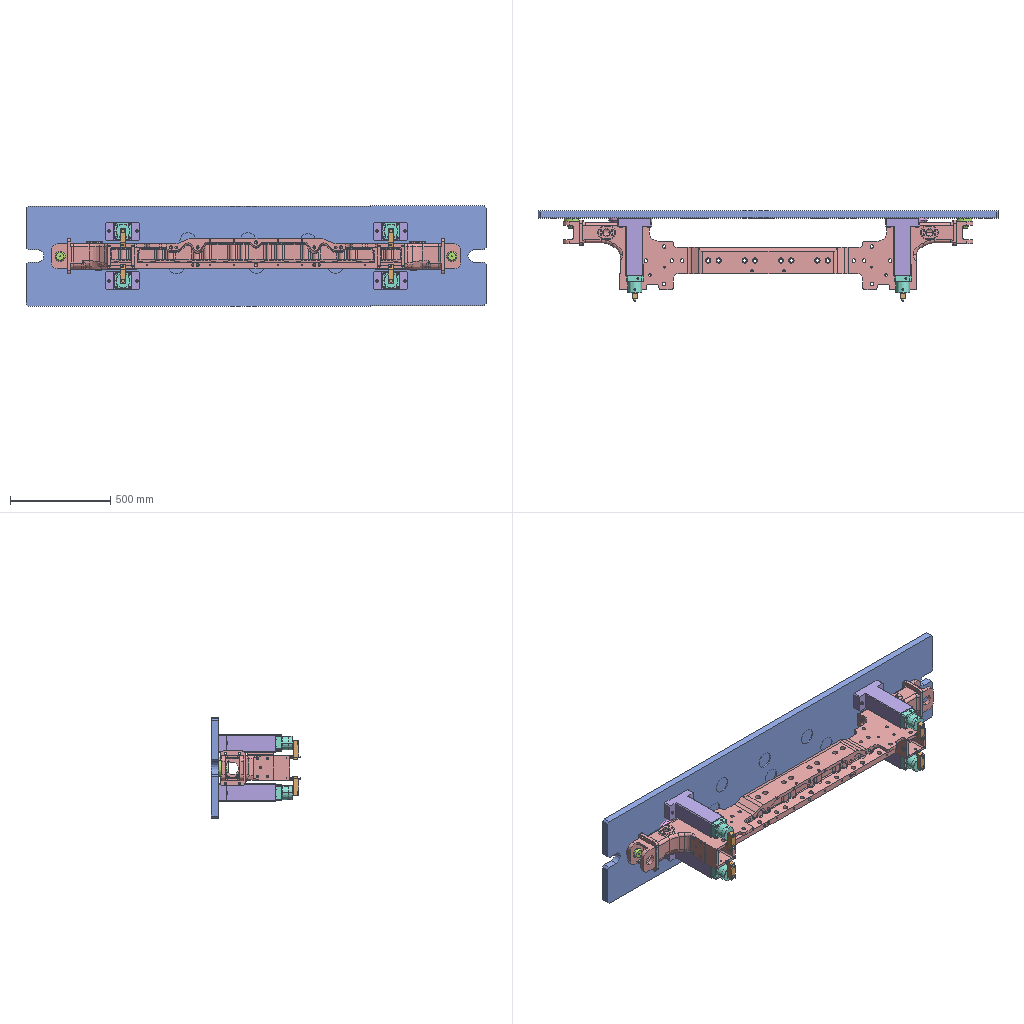Assembly | SolidWorks | 13 different items | 36 placed | box 2300 x 450 x 500 mm
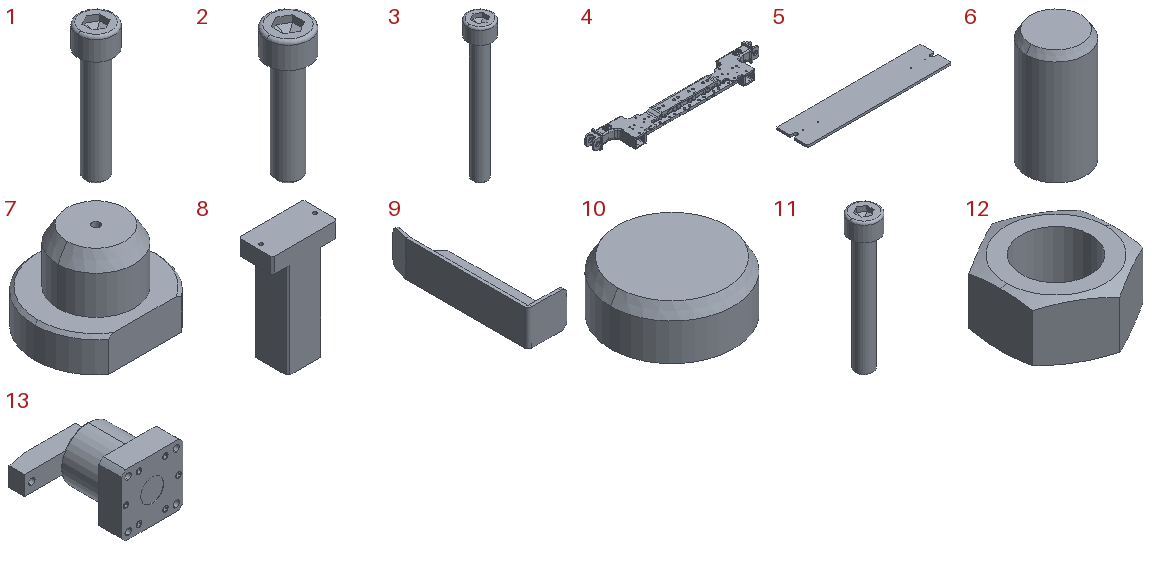Parts list (item | quantity | size | volume | features):
1 | x4 | 16 x 16 x 60 mm | 5707 mm3 | features Chamfer 2, Fillet 2, ICE 2, Extrusion 1, RefAxis 1
2 | x2 | 10 x 10 x 31 mm | 1125 mm3 | features Chamfer 2, Fillet 2, ICE 2, Extrusion 1, RefAxis 1
3 | x2 | 10 x 10 x 56 mm | 1832 mm3 | features Chamfer 2, Fillet 2, ICE 2, Extrusion 1, RefAxis 1
4 | x1 | 2048 x 348 x 175.5 mm | 20391465 mm3 | features ICE 2, BaseBody 1, DelFace 1
5 | x1 | 2300 x 500 x 35 mm | 39674536 mm3 | features ICE 3, Cut 2, HoleWzd 2, Chamfer 1, Extrusion 1
6 | x1 | 80 x 80 x 152 mm | 756529 mm3 | features Chamfer 1, Extrusion 1, HoleWzd 1
7 | x2 | 80 x 72 x 57 mm | 167700 mm3 | features Chamfer 2, ICE 2, Extrusion 1, HoleWzd 1
8 | x4 | 170 x 90 x 288 mm | 2601311 mm3 | features Chamfer 1, Extrusion 1, HoleWzd 1, ICE 1
9 | x1 | 65 x 235.272 x 60 mm | 126254 mm3 | features Fillet 1, FlatPattern 1, Gusset 1, SMBaseFlange 1, SheetMetal 1
10 | x2 | 100 x 100 x 40 mm | 304768 mm3 | features Chamfer 1, Extrusion 1, HoleWzd 1
11 | x8 | 13 x 13 x 63 mm | 3718 mm3 | features Chamfer 2, Fillet 2, ICE 2, Extrusion 1, RefAxis 1
12 | x4 | 16 x 18.475 x 8.4 mm | 1174 mm3 | features Extrusion 1, ICE 1, MirrorPattern 1, RefAxis 1, RevCut 1
13 | x4 | 121 x 115.5 x 82 mm | 382870 mm3 | features BaseBody 2, HoleWzd 1, ICE 1
Mates (type | each side: item.copy, entity, surface, feature):
Concentric | 4.1 face cylinder Input1 | 7.1 face cylinder Boss-Extrude1
Width | 4.1 face plane Input1 | 4.1 face plane Input1 | 5.1 face plane Boss-Extrude1 | 5.1 face plane Boss-Extrude1
Coincident | 4.1 face plane Input1 | 7.1 face plane Boss-Extrude2
Parallel | 4.1 face plane Input1 | 7.1 face plane Cut-Extrude1
Concentric | 4.1 face cylinder Input1 | 7.2 face cylinder Boss-Extrude1
Parallel | 4.1 face plane Input1 | 7.2 face plane Cut-Extrude1
Coincident | 4.1 face plane Input1 | 7.2 face plane Boss-Extrude2
Width | 5.1 face plane Boss-Extrude1 | 5.1 face plane Boss-Extrude1 | 4.1 face plane Input1 | 4.1 face plane Input1
Coincident | 5.1 face plane Cut-Extrude1 | 7.1 face plane Boss-Extrude2
Coincident | 4.1 face plane Input1 | 10.1 face plane Boss-Extrude1
Width | 4.1 face plane Input1 | 4.1 face plane Input1 | 10.1 face cylinder Boss-Extrude1
DistanceDim | 10.1 face cylinder Boss-Extrude1 | 4.1 face plane Input1
Width | 4.1 face plane Input1 | 4.1 face plane Input1 | 10.2 face cylinder Boss-Extrude1
DistanceDim | 10.2 face cylinder Boss-Extrude1 | 4.1 face plane Input1
Coincident | 4.1 face plane Input1 | 10.2 face plane Boss-Extrude1
Coincident | 4.1 face plane Input1 | 6.1 face
DistanceDim | 6.1 face | 4.1 face plane Input1 | 2 times
Coincident | 4.1 face plane Input1 | 6.2 face
DistanceDim | 6.2 face | 4.1 face plane Input1 | 2 times
Coincident | 4.1 face plane Input1 | 6.3 face
DistanceDim | 4.1 face plane Input1 | 6.3 face
Coincident | 4.1 face plane Input1 | 6.4 face
DistanceDim | 6.4 face | 4.1 face plane Input1
DistanceDim | 6.3 face | 6.2 face
DistanceDim | 6.3 face | 6.4 face
Coincident | 4.1 face plane Input1 | 6.5 face
DistanceDim | 4.1 face plane Input1 | 6.5 face
DistanceDim | 6.5 face | 4.1 face plane Input1
Coincident | 4.1 face plane Input1 | 6.6 face
DistanceDim | 6.6 face | 4.1 face plane Input1
DistanceDim | 6.6 face | 6.1 face
DistanceDim | 13.1 face plane _ACKx63_r-1-solid1 | 4.1 face plane Input1
Width | 4.1 face plane Input1 | 4.1 face plane Input1 | 13.1 face plane _ACKx63_r-1-solid1 | 13.1 face plane _ACKx63_r-1-solid1
Width | 4.1 face plane Input1 | 4.1 face plane Input1 | 13.2 face plane _ACKx63_r-1-solid1 | 13.2 face plane _ACKx63_r-1-solid1
DistanceDim | 13.2 face plane _ACKx63_r-1-solid1 | 4.1 face plane Input1
Coincident | 5.1 face plane Boss-Extrude1 | 8.1 face plane Boss-Extrude1
Width | 13.1 face plane _ACKx63_b-1-solid1 | 13.1 face plane _ACKx63_b-1-solid1 | 8.1 face plane Boss-Extrude1 | 8.1 face plane Boss-Extrude1 | 2 times
Coincident | 5.1 face plane Boss-Extrude1 | 8.2 face plane Boss-Extrude1
Width | 13.2 face plane _ACKx63_b-1-solid1 | 13.2 face plane _ACKx63_b-1-solid1 | 8.2 face plane Boss-Extrude1 | 8.2 face plane Boss-Extrude1 | 2 times
Coincident | 5.1 face plane Boss-Extrude1 | 9.1 face
DistanceDim | 9.1 face | 4.1 face plane Input1 | 2 times
Coincident | 5.1 face plane Boss-Extrude1 | 9.2 face
DistanceDim | 9.2 face | 4.1 face plane Input1
Coincident | 9.1 face | 9.2 face
Coincident | 5.1 face plane CBORE for M6 Hexagon socket head cap screws1 | 3.1 plane
Concentric | 7.1 face cylinder M6 Tapped Hole1 | 3.1 axis
Coincident | 5.1 face plane CBORE for M6 Hexagon socket head cap screws1 | 2.1 plane
Concentric | 10.1 face cylinder M6 Tapped Hole1 | 2.1 axis
Concentric | 7.2 face cylinder M6 Tapped Hole1 | 3.2 face cylinder Boss-Extrude2
Coincident | 5.1 face plane CBORE for M6 Hexagon socket head cap screws1 | 3.2 face plane Boss-Extrude1
Concentric | 5.1 face cylinder CBORE for M6 Hexagon socket head cap screws1 | 2.2 face cylinder Boss-Extrude2
Coincident | 5.1 face plane CBORE for M6 Hexagon socket head cap screws1 | 2.2 face plane Boss-Extrude1
Coincident | 8.3 face plane Boss-Extrude2 | 11.1 plane
Concentric | 5.1 face cylinder M8 Tapped Hole1 | 11.1 axis
Coincident | 8.3 face plane Boss-Extrude2 | 11.2 plane
Concentric | 5.1 face cylinder M8 Tapped Hole1 | 11.2 axis
Coincident | 8.3 face plane Boss-Extrude2 | 11.3 plane
Concentric | 5.1 face cylinder M8 Tapped Hole1 | 11.3 axis
Coincident | 8.3 face plane Boss-Extrude2 | 11.4 plane
Concentric | 5.1 face cylinder M8 Tapped Hole1 | 11.4 axis
Coincident | 8.3 face plane Boss-Extrude2 | 11.5 plane
Concentric | 5.1 face cylinder M8 Tapped Hole1 | 11.5 axis
Coincident | 8.3 face plane Boss-Extrude2 | 11.6 plane
Concentric | 5.1 face cylinder M8 Tapped Hole1 | 11.6 axis
Coincident | 8.3 face plane Boss-Extrude2 | 11.7 plane
Concentric | 5.1 face cylinder M8 Tapped Hole1 | 11.7 axis
Coincident | 8.3 face plane Boss-Extrude2 | 11.8 plane
Concentric | 5.1 face cylinder M8 Tapped Hole1 | 11.8 axis
Coincident | 13.1 face plane _ACKx63_r-1-solid1 | 12.1 plane
Concentric | 13.1 face cylinder M10 Tapped Hole1 | 1.1 axis
Coincident | 1.1 axis | 12.1 axis
DistanceDim | 1.1 face plane Boss-Extrude1 | 12.1 face plane Boss-Extrude1
Concentric | 13.2 face cylinder M10 Tapped Hole1 | 1.2 face cylinder Boss-Extrude2
Coincident | 1.1 face plane Boss-Extrude1 | 1.2 face plane Boss-Extrude1
Concentric | 1.2 face cylinder Boss-Extrude2 | 12.2 face cylinder Cut-Extrude1
Coincident | 13.2 face plane _ACKx63_r-1-solid1 | 12.2 face plane Boss-Extrude1
Coincident | 13.1 face plane _ACKx63_b-1-solid1 | 8.1 face plane Boss-Extrude1
Coincident | 13.2 face plane _ACKx63_b-1-solid1 | 8.2 face plane Boss-Extrude1